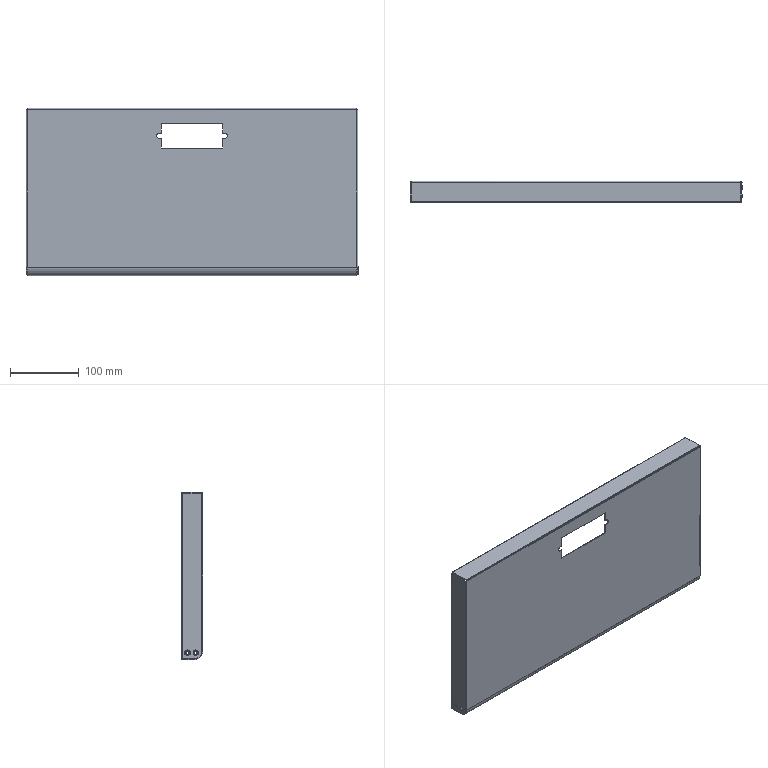Part | NX | features BREP 13 | 13 solids | 400 faces | box 484 x 31 x 244 mm | volume 170539 mm3 | plane 154 | cylinder 122 | cone 112 | spline 12 | commonest cylinder face diameters 8 x48 3.3 x16 4.5 x16 4.134 x8 5.5 x8 1.473 x7